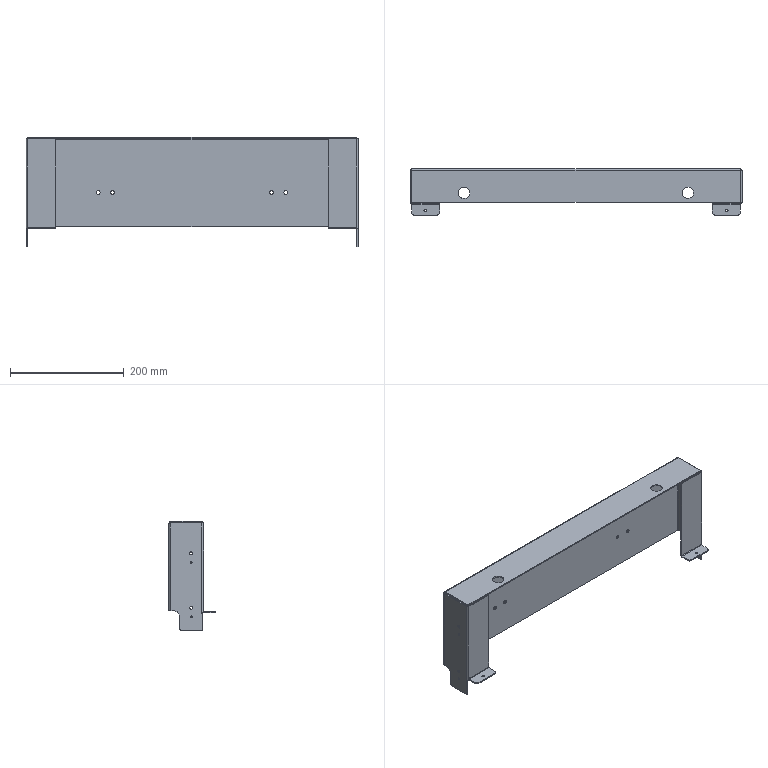Part | NX | 1 solid | 100 faces | box 584 x 81 x 192 mm | volume 322950 mm3 | plane 58 | cylinder 38 | spline 4 | commonest cylinder face diameters 2 x7 6 x7 5 x6 10 x6 3.3 x4 6.6 x4